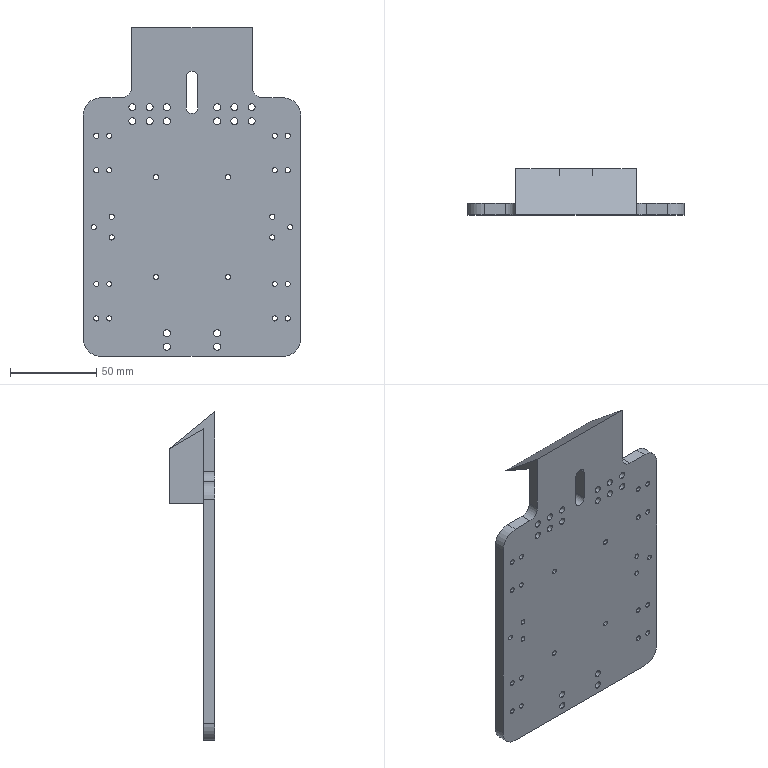Part | SolidWorks | features ICE 8, MirrorPattern 5, Fillet 2, Extrusion 1 | 1 solid | 111 faces | box 126 x 26.5 x 190.71 mm | volume 150681 mm3 | cylinder 93 | plane 18 | commonest cylinder face diameters 3 x52 4 x32 20 x4 6.772 x3 12 x2